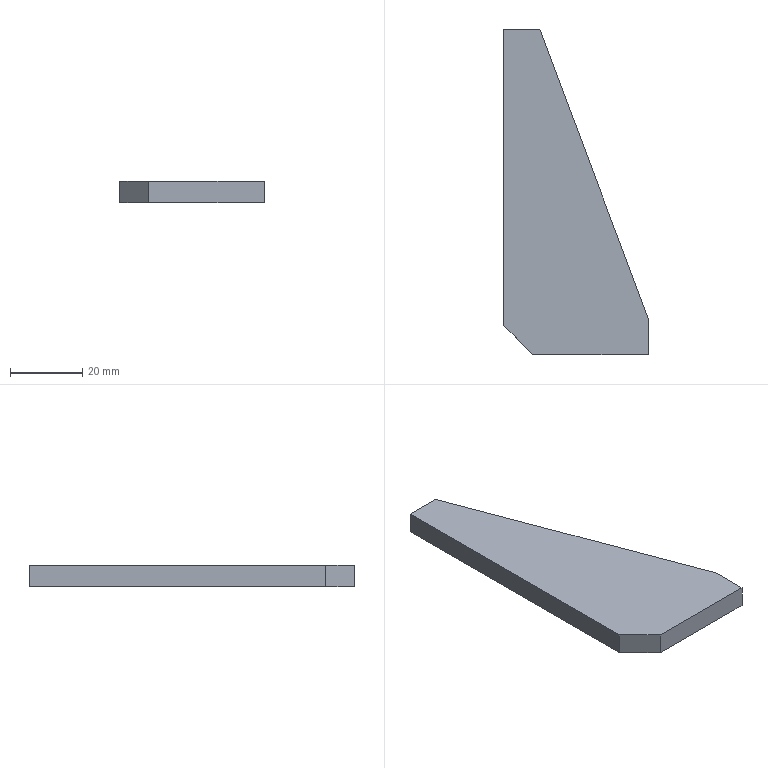Part | SolidWorks | features Chamfer 1, Extrusion 1 | 1 solid | 8 faces | box 40 x 90 x 6 mm | volume 14208 mm3 | plane 8
STEP:
#1=CARTESIAN_POINT('',(10.,90.,-3.));
#2=VERTEX_POINT('',#1);
#3=CARTESIAN_POINT('',(0.,90.,-3.));
#4=VERTEX_POINT('',#3);
#5=CARTESIAN_POINT('',(10.,90.,-3.));
#6=DIRECTION('',(-1.,0.,0.));
#7=VECTOR('',#6,1000.);
#8=LINE('',#5,#7);
#9=EDGE_CURVE('',#2,#4,#8,.T.);
#10=ORIENTED_EDGE('',*,*,#9,.T.);
#11=CARTESIAN_POINT('',(0.,90.,3.));
#12=VERTEX_POINT('',#11);
#13=CARTESIAN_POINT('',(0.,90.,3.));
#14=DIRECTION('',(0.,0.,-1.));
#15=VECTOR('',#14,1000.);
#16=LINE('',#13,#15);
#17=EDGE_CURVE('',#12,#4,#16,.T.);
#18=ORIENTED_EDGE('',*,*,#17,.F.);
#19=CARTESIAN_POINT('',(10.,90.,3.));
#20=VERTEX_POINT('',#19);
#21=CARTESIAN_POINT('',(10.,90.,3.));
#22=DIRECTION('',(-1.,0.,0.));
#23=VECTOR('',#22,1000.);
#24=LINE('',#21,#23);
#25=EDGE_CURVE('',#20,#12,#24,.T.);
#26=ORIENTED_EDGE('',*,*,#25,.F.);
#27=CARTESIAN_POINT('',(10.,90.,3.));
#28=DIRECTION('',(0.,0.,-1.));
#29=VECTOR('',#28,1000.);
#30=LINE('',#27,#29);
#31=EDGE_CURVE('',#20,#2,#30,.T.);
#32=ORIENTED_EDGE('',*,*,#31,.T.);
#33=EDGE_LOOP('',(#10,#18,#26,#32));
#34=FACE_OUTER_BOUND('',#33,.T.);
#35=CARTESIAN_POINT('',(10.,90.,3.));
#36=DIRECTION('',(0.,-1.,0.));
#37=DIRECTION('',(1.,0.,0.));
#38=AXIS2_PLACEMENT_3D('',#35,#36,#37);
#39=PLANE('',#38);
#40=ADVANCED_FACE('',(#34),#39,.F.);
#41=CARTESIAN_POINT('',(0.,8.,-3.));
#42=VERTEX_POINT('',#41);
#43=CARTESIAN_POINT('',(0.,90.,-3.));
#44=DIRECTION('',(0.,-1.,0.));
#45=VECTOR('',#44,1000.);
#46=LINE('',#43,#45);
#47=EDGE_CURVE('',#4,#42,#46,.T.);
#48=ORIENTED_EDGE('',*,*,#47,.T.);
#49=CARTESIAN_POINT('',(0.,8.,3.));
#50=VERTEX_POINT('',#49);
#51=CARTESIAN_POINT('',(0.,8.,3.));
#52=DIRECTION('',(0.,0.,1.));
#53=VECTOR('',#52,1000.);
#54=LINE('',#51,#53);
#55=EDGE_CURVE('',#42,#50,#54,.T.);
#56=ORIENTED_EDGE('',*,*,#55,.T.);
#57=CARTESIAN_POINT('',(0.,90.,3.));
#58=DIRECTION('',(0.,-1.,0.));
#59=VECTOR('',#58,1000.);
#60=LINE('',#57,#59);
#61=EDGE_CURVE('',#12,#50,#60,.T.);
#62=ORIENTED_EDGE('',*,*,#61,.F.);
#63=ORIENTED_EDGE('',*,*,#17,.T.);
#64=EDGE_LOOP('',(#48,#56,#62,#63));
#65=FACE_OUTER_BOUND('',#64,.T.);
#66=CARTESIAN_POINT('',(0.,90.,3.));
#67=DIRECTION('',(1.,0.,0.));
#68=DIRECTION('',(0.,1.,0.));
#69=AXIS2_PLACEMENT_3D('',#66,#67,#68);
#70=PLANE('',#69);
#71=ADVANCED_FACE('',(#65),#70,.F.);
#72=CARTESIAN_POINT('',(8.,0.,3.));
#73=VERTEX_POINT('',#72);
#74=CARTESIAN_POINT('',(40.,0.,3.));
#75=VERTEX_POINT('',#74);
#76=CARTESIAN_POINT('',(0.,0.,3.));
#77=DIRECTION('',(1.,0.,0.));
#78=VECTOR('',#77,1000.);
#79=LINE('',#76,#78);
#80=EDGE_CURVE('',#73,#75,#79,.T.);
#81=ORIENTED_EDGE('',*,*,#80,.F.);
#82=CARTESIAN_POINT('',(8.,0.,-3.));
#83=VERTEX_POINT('',#82);
#84=CARTESIAN_POINT('',(8.,0.,3.));
#85=DIRECTION('',(0.,0.,-1.));
#86=VECTOR('',#85,1000.);
#87=LINE('',#84,#86);
#88=EDGE_CURVE('',#73,#83,#87,.T.);
#89=ORIENTED_EDGE('',*,*,#88,.T.);
#90=CARTESIAN_POINT('',(40.,0.,-3.));
#91=VERTEX_POINT('',#90);
#92=CARTESIAN_POINT('',(0.,0.,-3.));
#93=DIRECTION('',(1.,0.,0.));
#94=VECTOR('',#93,1000.);
#95=LINE('',#92,#94);
#96=EDGE_CURVE('',#83,#91,#95,.T.);
#97=ORIENTED_EDGE('',*,*,#96,.T.);
#98=CARTESIAN_POINT('',(40.,0.,3.));
#99=DIRECTION('',(0.,0.,-1.));
#100=VECTOR('',#99,1000.);
#101=LINE('',#98,#100);
#102=EDGE_CURVE('',#75,#91,#101,.T.);
#103=ORIENTED_EDGE('',*,*,#102,.F.);
#104=EDGE_LOOP('',(#81,#89,#97,#103));
#105=FACE_OUTER_BOUND('',#104,.T.);
#106=CARTESIAN_POINT('',(0.,0.,3.));
#107=DIRECTION('',(0.,1.,0.));
#108=DIRECTION('',(0.,0.,1.));
#109=AXIS2_PLACEMENT_3D('',#106,#107,#108);
#110=PLANE('',#109);
#111=ADVANCED_FACE('',(#105),#110,.F.);
#112=CARTESIAN_POINT('',(40.,10.,-3.));
#113=VERTEX_POINT('',#112);
#114=CARTESIAN_POINT('',(40.,0.,-3.));
#115=DIRECTION('',(0.,1.,0.));
#116=VECTOR('',#115,1000.);
#117=LINE('',#114,#116);
#118=EDGE_CURVE('',#91,#113,#117,.T.);
#119=ORIENTED_EDGE('',*,*,#118,.T.);
#120=CARTESIAN_POINT('',(40.,10.,3.));
#121=VERTEX_POINT('',#120);
#122=CARTESIAN_POINT('',(40.,10.,3.));
#123=DIRECTION('',(0.,0.,-1.));
#124=VECTOR('',#123,1000.);
#125=LINE('',#122,#124);
#126=EDGE_CURVE('',#121,#113,#125,.T.);
#127=ORIENTED_EDGE('',*,*,#126,.F.);
#128=CARTESIAN_POINT('',(40.,0.,3.));
#129=DIRECTION('',(0.,1.,0.));
#130=VECTOR('',#129,1000.);
#131=LINE('',#128,#130);
#132=EDGE_CURVE('',#75,#121,#131,.T.);
#133=ORIENTED_EDGE('',*,*,#132,.F.);
#134=ORIENTED_EDGE('',*,*,#102,.T.);
#135=EDGE_LOOP('',(#119,#127,#133,#134));
#136=FACE_OUTER_BOUND('',#135,.T.);
#137=CARTESIAN_POINT('',(40.,0.,3.));
#138=DIRECTION('',(-1.,0.,0.));
#139=DIRECTION('',(0.,0.,1.));
#140=AXIS2_PLACEMENT_3D('',#137,#138,#139);
#141=PLANE('',#140);
#142=ADVANCED_FACE('',(#136),#141,.F.);
#143=CARTESIAN_POINT('',(40.,10.,-3.));
#144=DIRECTION('',(-0.3511,0.9363,0.));
#145=VECTOR('',#144,1000.);
#146=LINE('',#143,#145);
#147=EDGE_CURVE('',#113,#2,#146,.T.);
#148=ORIENTED_EDGE('',*,*,#147,.T.);
#149=ORIENTED_EDGE('',*,*,#31,.F.);
#150=CARTESIAN_POINT('',(40.,10.,3.));
#151=DIRECTION('',(-0.3511,0.9363,0.));
#152=VECTOR('',#151,1000.);
#153=LINE('',#150,#152);
#154=EDGE_CURVE('',#121,#20,#153,.T.);
#155=ORIENTED_EDGE('',*,*,#154,.F.);
#156=ORIENTED_EDGE('',*,*,#126,.T.);
#157=EDGE_LOOP('',(#148,#149,#155,#156));
#158=FACE_OUTER_BOUND('',#157,.T.);
#159=CARTESIAN_POINT('',(40.,10.,3.));
#160=DIRECTION('',(-0.9363,-0.3511,0.));
#161=DIRECTION('',(0.3511,-0.9363,0.));
#162=AXIS2_PLACEMENT_3D('',#159,#160,#161);
#163=PLANE('',#162);
#164=ADVANCED_FACE('',(#158),#163,.F.);
#165=ORIENTED_EDGE('',*,*,#61,.T.);
#166=CARTESIAN_POINT('',(4.,4.,3.));
#167=DIRECTION('',(0.7071,-0.7071,0.));
#168=VECTOR('',#167,1000.);
#169=LINE('',#166,#168);
#170=EDGE_CURVE('',#50,#73,#169,.T.);
#171=ORIENTED_EDGE('',*,*,#170,.T.);
#172=ORIENTED_EDGE('',*,*,#80,.T.);
#173=ORIENTED_EDGE('',*,*,#132,.T.);
#174=ORIENTED_EDGE('',*,*,#154,.T.);
#175=ORIENTED_EDGE('',*,*,#25,.T.);
#176=EDGE_LOOP('',(#165,#171,#172,#173,#174,#175));
#177=FACE_OUTER_BOUND('',#176,.T.);
#178=CARTESIAN_POINT('',(0.,0.,3.));
#179=DIRECTION('',(0.,0.,1.));
#180=DIRECTION('',(1.,0.,0.));
#181=AXIS2_PLACEMENT_3D('',#178,#179,#180);
#182=PLANE('',#181);
#183=ADVANCED_FACE('',(#177),#182,.T.);
#184=ORIENTED_EDGE('',*,*,#96,.F.);
#185=CARTESIAN_POINT('',(8.,0.,-3.));
#186=DIRECTION('',(-0.7071,0.7071,0.));
#187=VECTOR('',#186,1000.);
#188=LINE('',#185,#187);
#189=EDGE_CURVE('',#83,#42,#188,.T.);
#190=ORIENTED_EDGE('',*,*,#189,.T.);
#191=ORIENTED_EDGE('',*,*,#47,.F.);
#192=ORIENTED_EDGE('',*,*,#9,.F.);
#193=ORIENTED_EDGE('',*,*,#147,.F.);
#194=ORIENTED_EDGE('',*,*,#118,.F.);
#195=EDGE_LOOP('',(#184,#190,#191,#192,#193,#194));
#196=FACE_OUTER_BOUND('',#195,.T.);
#197=CARTESIAN_POINT('',(0.,0.,-3.));
#198=DIRECTION('',(0.,0.,1.));
#199=DIRECTION('',(1.,0.,0.));
#200=AXIS2_PLACEMENT_3D('',#197,#198,#199);
#201=PLANE('',#200);
#202=ADVANCED_FACE('',(#196),#201,.F.);
#203=ORIENTED_EDGE('',*,*,#170,.F.);
#204=ORIENTED_EDGE('',*,*,#55,.F.);
#205=ORIENTED_EDGE('',*,*,#189,.F.);
#206=ORIENTED_EDGE('',*,*,#88,.F.);
#207=EDGE_LOOP('',(#203,#204,#205,#206));
#208=FACE_OUTER_BOUND('',#207,.T.);
#209=CARTESIAN_POINT('',(8.,0.,3.));
#210=DIRECTION('',(0.7071,0.7071,0.));
#211=DIRECTION('',(0.,0.,-1.));
#212=AXIS2_PLACEMENT_3D('',#209,#210,#211);
#213=PLANE('',#212);
#214=ADVANCED_FACE('',(#208),#213,.F.);
#215=CLOSED_SHELL('',(#40,#71,#111,#142,#164,#183,#202,#214));
#216=MANIFOLD_SOLID_BREP('',#215);
#217=CARTESIAN_POINT('',(0.,0.,0.));
#218=DIRECTION('',(0.,0.,1.));
#219=DIRECTION('',(1.,0.,0.));
#220=AXIS2_PLACEMENT_3D('',#217,#218,#219);
#221=(LENGTH_UNIT()NAMED_UNIT(*)SI_UNIT(.MILLI.,.METRE.));
#222=UNCERTAINTY_MEASURE_WITH_UNIT(LENGTH_MEASURE(0.00001),#221,'','');
#223=(NAMED_UNIT(*)PLANE_ANGLE_UNIT()SI_UNIT($,.RADIAN.));
#224=(NAMED_UNIT(*)SI_UNIT($,.STERADIAN.)SOLID_ANGLE_UNIT());
#225=(GEOMETRIC_REPRESENTATION_CONTEXT(3)GLOBAL_UNCERTAINTY_ASSIGNED_CONTEXT((#222))GLOBAL_UNIT_ASSIGNED_CONTEXT((#221,#223,#224))REPRESENTATION_CONTEXT('',''));
#226=ADVANCED_BREP_SHAPE_REPRESENTATION('',(#216,#220),#225);